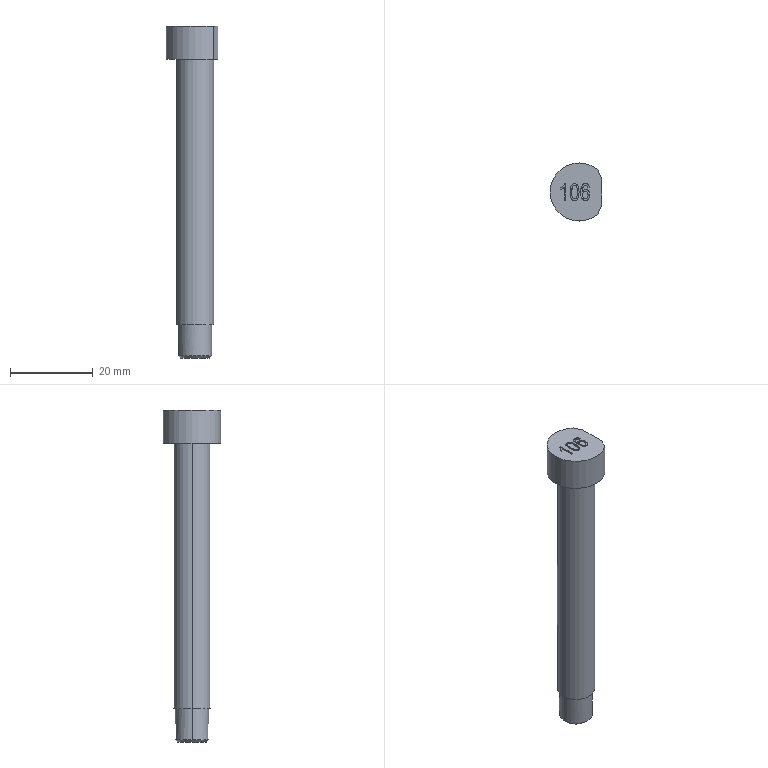Part | Creo | 1 solid | 55 faces | box 12.5 x 14 x 80.193 mm | volume 5631 mm3 | other 30 | plane 18 | cylinder 5 | cone 2 | commonest cylinder face diameters 8 x2 9 x2 14 x1